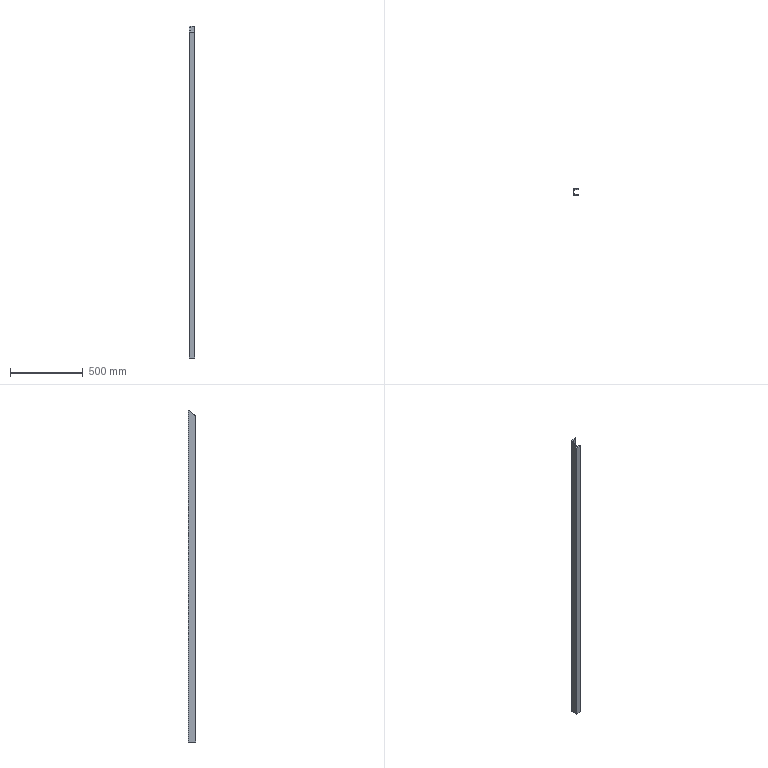Part | STEP file | DIN 1026-1 U 50 1785357157092 | 1 solid | 14 faces | box 38 x 50 x 2278 mm | volume 1606422 mm3 | plane 10 | cylinder 4 | commonest cylinder face diameters 7 x2 14 x2
STEP:
#1=CARTESIAN_POINT('',(5.,-10.418,2334.303));
#2=VERTEX_POINT('',#1);
#3=CARTESIAN_POINT('',(11.442,-17.395,2328.445));
#4=VERTEX_POINT('',#3);
#5=CARTESIAN_POINT('',(12.,-10.418,2334.303));
#6=DIRECTION('',(0.,-0.643,0.7659));
#7=DIRECTION('',(0.,-0.7659,-0.643));
#8=AXIS2_PLACEMENT_3D('',#5,#6,#7);
#9=ELLIPSE('',#8,9.14,7.);
#10=EDGE_CURVE('',#2,#4,#9,.T.);
#11=ORIENTED_EDGE('',*,*,#10,.F.);
#12=CARTESIAN_POINT('',(5.,10.418,2351.795));
#13=VERTEX_POINT('',#12);
#14=CARTESIAN_POINT('',(5.,-1153.83,1374.368));
#15=DIRECTION('',(0.,-0.7659,-0.643));
#16=VECTOR('',#15,10.);
#17=LINE('',#14,#16);
#18=EDGE_CURVE('',#13,#2,#17,.T.);
#19=ORIENTED_EDGE('',*,*,#18,.F.);
#20=CARTESIAN_POINT('',(11.442,17.395,2357.653));
#21=VERTEX_POINT('',#20);
#22=CARTESIAN_POINT('',(12.,10.418,2351.795));
#23=DIRECTION('',(0.,-0.643,0.7659));
#24=DIRECTION('',(0.,0.7659,0.643));
#25=AXIS2_PLACEMENT_3D('',#22,#23,#24);
#26=ELLIPSE('',#25,9.14,7.);
#27=EDGE_CURVE('',#21,#13,#26,.T.);
#28=ORIENTED_EDGE('',*,*,#27,.F.);
#29=CARTESIAN_POINT('',(34.779,19.262,2359.22));
#30=VERTEX_POINT('',#29);
#31=CARTESIAN_POINT('',(-139.927,5.286,2347.486));
#32=DIRECTION('',(-0.9946,-0.07957,-0.0668));
#33=VECTOR('',#32,10.);
#34=LINE('',#31,#33);
#35=EDGE_CURVE('',#30,#21,#34,.T.);
#36=ORIENTED_EDGE('',*,*,#35,.F.);
#37=CARTESIAN_POINT('',(38.,22.751,2362.149));
#38=VERTEX_POINT('',#37);
#39=CARTESIAN_POINT('',(34.5,22.751,2362.149));
#40=DIRECTION('',(0.,0.643,-0.7659));
#41=DIRECTION('',(0.,0.7659,0.643));
#42=AXIS2_PLACEMENT_3D('',#39,#40,#41);
#43=ELLIPSE('',#42,4.57,3.5);
#44=EDGE_CURVE('',#38,#30,#43,.T.);
#45=ORIENTED_EDGE('',*,*,#44,.F.);
#46=CARTESIAN_POINT('',(38.,25.,2364.037));
#47=VERTEX_POINT('',#46);
#48=CARTESIAN_POINT('',(38.,-1146.498,1380.523));
#49=DIRECTION('',(0.,-0.7659,-0.643));
#50=VECTOR('',#49,10.);
#51=LINE('',#48,#50);
#52=EDGE_CURVE('',#47,#38,#51,.T.);
#53=ORIENTED_EDGE('',*,*,#52,.F.);
#54=CARTESIAN_POINT('',(0.,25.,2364.037));
#55=VERTEX_POINT('',#54);
#56=CARTESIAN_POINT('',(9.5,25.,2364.037));
#57=DIRECTION('',(1.,0.,0.));
#58=VECTOR('',#57,10.);
#59=LINE('',#56,#58);
#60=EDGE_CURVE('',#55,#47,#59,.T.);
#61=ORIENTED_EDGE('',*,*,#60,.F.);
#62=CARTESIAN_POINT('',(0.,-25.,2322.06));
#63=VERTEX_POINT('',#62);
#64=CARTESIAN_POINT('',(0.,-1153.83,1374.368));
#65=DIRECTION('',(0.,0.7659,0.643));
#66=VECTOR('',#65,10.);
#67=LINE('',#64,#66);
#68=EDGE_CURVE('',#63,#55,#67,.T.);
#69=ORIENTED_EDGE('',*,*,#68,.F.);
#70=CARTESIAN_POINT('',(38.,-25.,2322.06));
#71=VERTEX_POINT('',#70);
#72=CARTESIAN_POINT('',(19.,-25.,2322.06));
#73=DIRECTION('',(-1.,0.,0.));
#74=VECTOR('',#73,10.);
#75=LINE('',#72,#74);
#76=EDGE_CURVE('',#71,#63,#75,.T.);
#77=ORIENTED_EDGE('',*,*,#76,.F.);
#78=CARTESIAN_POINT('',(38.,-22.751,2323.948));
#79=VERTEX_POINT('',#78);
#80=CARTESIAN_POINT('',(38.,-1160.503,1368.766));
#81=DIRECTION('',(0.,-0.7659,-0.643));
#82=VECTOR('',#81,10.);
#83=LINE('',#80,#82);
#84=EDGE_CURVE('',#79,#71,#83,.T.);
#85=ORIENTED_EDGE('',*,*,#84,.F.);
#86=CARTESIAN_POINT('',(34.779,-19.262,2326.877));
#87=VERTEX_POINT('',#86);
#88=CARTESIAN_POINT('',(34.5,-22.751,2323.948));
#89=DIRECTION('',(0.,0.643,-0.7659));
#90=DIRECTION('',(0.,-0.7659,-0.643));
#91=AXIS2_PLACEMENT_3D('',#88,#89,#90);
#92=ELLIPSE('',#91,4.57,3.5);
#93=EDGE_CURVE('',#87,#79,#92,.T.);
#94=ORIENTED_EDGE('',*,*,#93,.F.);
#95=CARTESIAN_POINT('',(159.791,-29.263,2318.481));
#96=DIRECTION('',(0.9946,-0.07957,-0.0668));
#97=VECTOR('',#96,10.);
#98=LINE('',#95,#97);
#99=EDGE_CURVE('',#4,#87,#98,.T.);
#100=ORIENTED_EDGE('',*,*,#99,.F.);
#101=EDGE_LOOP('',(#11,#19,#28,#36,#45,#53,#61,#69,#77,#85,#94,#100));
#102=FACE_OUTER_BOUND('',#101,.T.);
#103=CARTESIAN_POINT('',(0.,-1153.83,1374.368));
#104=DIRECTION('',(0.,0.643,-0.7659));
#105=DIRECTION('',(-1.,0.,0.));
#106=AXIS2_PLACEMENT_3D('',#103,#104,#105);
#107=PLANE('',#106);
#108=ADVANCED_FACE('',(#102),#107,.F.);
#109=ORIENTED_EDGE('',*,*,#52,.T.);
#110=CARTESIAN_POINT('',(38.,22.751,86.4));
#111=VERTEX_POINT('',#110);
#112=CARTESIAN_POINT('',(38.,22.751,0.));
#113=DIRECTION('',(0.,0.,1.));
#114=VECTOR('',#113,10.);
#115=LINE('',#112,#114);
#116=EDGE_CURVE('',#111,#38,#115,.T.);
#117=ORIENTED_EDGE('',*,*,#116,.F.);
#118=CARTESIAN_POINT('',(38.,25.,86.4));
#119=VERTEX_POINT('',#118);
#120=CARTESIAN_POINT('',(38.,12.5,86.4));
#121=DIRECTION('',(0.,-1.,0.));
#122=VECTOR('',#121,10.);
#123=LINE('',#120,#122);
#124=EDGE_CURVE('',#119,#111,#123,.T.);
#125=ORIENTED_EDGE('',*,*,#124,.F.);
#126=CARTESIAN_POINT('',(38.,25.,0.));
#127=DIRECTION('',(0.,0.,1.));
#128=VECTOR('',#127,10.);
#129=LINE('',#126,#128);
#130=EDGE_CURVE('',#119,#47,#129,.T.);
#131=ORIENTED_EDGE('',*,*,#130,.T.);
#132=EDGE_LOOP('',(#109,#117,#125,#131));
#133=FACE_OUTER_BOUND('',#132,.T.);
#134=CARTESIAN_POINT('',(38.,25.,0.));
#135=DIRECTION('',(1.,0.,0.));
#136=DIRECTION('',(0.,0.,-1.));
#137=AXIS2_PLACEMENT_3D('',#134,#135,#136);
#138=PLANE('',#137);
#139=ADVANCED_FACE('',(#133),#138,.T.);
#140=ORIENTED_EDGE('',*,*,#44,.T.);
#141=CARTESIAN_POINT('',(34.779,19.262,86.4));
#142=VERTEX_POINT('',#141);
#143=CARTESIAN_POINT('',(34.779,19.262,0.));
#144=DIRECTION('',(0.,0.,1.));
#145=VECTOR('',#144,10.);
#146=LINE('',#143,#145);
#147=EDGE_CURVE('',#142,#30,#146,.T.);
#148=ORIENTED_EDGE('',*,*,#147,.F.);
#149=CARTESIAN_POINT('',(34.5,22.751,86.4));
#150=DIRECTION('',(0.,0.,-1.));
#151=DIRECTION('',(-0.07975,0.9968,0.));
#152=AXIS2_PLACEMENT_3D('',#149,#150,#151);
#153=CIRCLE('',#152,3.5);
#154=EDGE_CURVE('',#111,#142,#153,.T.);
#155=ORIENTED_EDGE('',*,*,#154,.F.);
#156=ORIENTED_EDGE('',*,*,#116,.T.);
#157=EDGE_LOOP('',(#140,#148,#155,#156));
#158=FACE_OUTER_BOUND('',#157,.T.);
#159=CARTESIAN_POINT('',(34.5,22.751,0.));
#160=DIRECTION('',(0.,0.,1.));
#161=DIRECTION('',(-0.07975,0.9968,0.));
#162=AXIS2_PLACEMENT_3D('',#159,#160,#161);
#163=CYLINDRICAL_SURFACE('',#162,3.5);
#164=ADVANCED_FACE('',(#158),#163,.T.);
#165=ORIENTED_EDGE('',*,*,#35,.T.);
#166=CARTESIAN_POINT('',(11.442,17.395,86.4));
#167=VERTEX_POINT('',#166);
#168=CARTESIAN_POINT('',(11.442,17.395,0.));
#169=DIRECTION('',(0.,0.,1.));
#170=VECTOR('',#169,10.);
#171=LINE('',#168,#170);
#172=EDGE_CURVE('',#167,#21,#171,.T.);
#173=ORIENTED_EDGE('',*,*,#172,.F.);
#174=CARTESIAN_POINT('',(26.174,18.574,86.4));
#175=DIRECTION('',(-0.9968,-0.07975,0.));
#176=VECTOR('',#175,10.);
#177=LINE('',#174,#176);
#178=EDGE_CURVE('',#142,#167,#177,.T.);
#179=ORIENTED_EDGE('',*,*,#178,.F.);
#180=ORIENTED_EDGE('',*,*,#147,.T.);
#181=EDGE_LOOP('',(#165,#173,#179,#180));
#182=FACE_OUTER_BOUND('',#181,.T.);
#183=CARTESIAN_POINT('',(34.779,19.262,0.));
#184=DIRECTION('',(0.07975,-0.9968,0.));
#185=DIRECTION('',(0.,0.,-1.));
#186=AXIS2_PLACEMENT_3D('',#183,#184,#185);
#187=PLANE('',#186);
#188=ADVANCED_FACE('',(#182),#187,.T.);
#189=ORIENTED_EDGE('',*,*,#27,.T.);
#190=CARTESIAN_POINT('',(5.,10.418,86.4));
#191=VERTEX_POINT('',#190);
#192=CARTESIAN_POINT('',(5.,10.418,0.));
#193=DIRECTION('',(0.,0.,1.));
#194=VECTOR('',#193,10.);
#195=LINE('',#192,#194);
#196=EDGE_CURVE('',#191,#13,#195,.T.);
#197=ORIENTED_EDGE('',*,*,#196,.F.);
#198=CARTESIAN_POINT('',(12.,10.418,86.4));
#199=DIRECTION('',(0.,0.,1.));
#200=DIRECTION('',(-0.07975,0.9968,0.));
#201=AXIS2_PLACEMENT_3D('',#198,#199,#200);
#202=CIRCLE('',#201,7.);
#203=EDGE_CURVE('',#167,#191,#202,.T.);
#204=ORIENTED_EDGE('',*,*,#203,.F.);
#205=ORIENTED_EDGE('',*,*,#172,.T.);
#206=EDGE_LOOP('',(#189,#197,#204,#205));
#207=FACE_OUTER_BOUND('',#206,.T.);
#208=CARTESIAN_POINT('',(12.,10.418,0.));
#209=DIRECTION('',(0.,0.,1.));
#210=DIRECTION('',(-0.07975,0.9968,0.));
#211=AXIS2_PLACEMENT_3D('',#208,#209,#210);
#212=CYLINDRICAL_SURFACE('',#211,7.);
#213=ADVANCED_FACE('',(#207),#212,.F.);
#214=ORIENTED_EDGE('',*,*,#18,.T.);
#215=CARTESIAN_POINT('',(5.,-10.418,86.4));
#216=VERTEX_POINT('',#215);
#217=CARTESIAN_POINT('',(5.,-10.418,0.));
#218=DIRECTION('',(0.,0.,1.));
#219=VECTOR('',#218,10.);
#220=LINE('',#217,#219);
#221=EDGE_CURVE('',#216,#2,#220,.T.);
#222=ORIENTED_EDGE('',*,*,#221,.F.);
#223=CARTESIAN_POINT('',(5.,0.,86.4));
#224=DIRECTION('',(0.,-1.,0.));
#225=VECTOR('',#224,10.);
#226=LINE('',#223,#225);
#227=EDGE_CURVE('',#191,#216,#226,.T.);
#228=ORIENTED_EDGE('',*,*,#227,.F.);
#229=ORIENTED_EDGE('',*,*,#196,.T.);
#230=EDGE_LOOP('',(#214,#222,#228,#229));
#231=FACE_OUTER_BOUND('',#230,.T.);
#232=CARTESIAN_POINT('',(5.,0.,0.));
#233=DIRECTION('',(1.,0.,0.));
#234=DIRECTION('',(0.,0.,-1.));
#235=AXIS2_PLACEMENT_3D('',#232,#233,#234);
#236=PLANE('',#235);
#237=ADVANCED_FACE('',(#231),#236,.T.);
#238=ORIENTED_EDGE('',*,*,#10,.T.);
#239=CARTESIAN_POINT('',(11.442,-17.395,86.4));
#240=VERTEX_POINT('',#239);
#241=CARTESIAN_POINT('',(11.442,-17.395,0.));
#242=DIRECTION('',(0.,0.,1.));
#243=VECTOR('',#242,10.);
#244=LINE('',#241,#243);
#245=EDGE_CURVE('',#240,#4,#244,.T.);
#246=ORIENTED_EDGE('',*,*,#245,.F.);
#247=CARTESIAN_POINT('',(12.,-10.418,86.4));
#248=DIRECTION('',(0.,0.,1.));
#249=DIRECTION('',(-1.,0.,0.));
#250=AXIS2_PLACEMENT_3D('',#247,#248,#249);
#251=CIRCLE('',#250,7.);
#252=EDGE_CURVE('',#216,#240,#251,.T.);
#253=ORIENTED_EDGE('',*,*,#252,.F.);
#254=ORIENTED_EDGE('',*,*,#221,.T.);
#255=EDGE_LOOP('',(#238,#246,#253,#254));
#256=FACE_OUTER_BOUND('',#255,.T.);
#257=CARTESIAN_POINT('',(12.,-10.418,0.));
#258=DIRECTION('',(0.,0.,1.));
#259=DIRECTION('',(-1.,0.,0.));
#260=AXIS2_PLACEMENT_3D('',#257,#258,#259);
#261=CYLINDRICAL_SURFACE('',#260,7.);
#262=ADVANCED_FACE('',(#256),#261,.F.);
#263=ORIENTED_EDGE('',*,*,#99,.T.);
#264=CARTESIAN_POINT('',(34.779,-19.262,86.4));
#265=VERTEX_POINT('',#264);
#266=CARTESIAN_POINT('',(34.779,-19.262,0.));
#267=DIRECTION('',(0.,0.,1.));
#268=VECTOR('',#267,10.);
#269=LINE('',#266,#268);
#270=EDGE_CURVE('',#265,#87,#269,.T.);
#271=ORIENTED_EDGE('',*,*,#270,.F.);
#272=CARTESIAN_POINT('',(14.505,-17.64,86.4));
#273=DIRECTION('',(0.9968,-0.07975,0.));
#274=VECTOR('',#273,10.);
#275=LINE('',#272,#274);
#276=EDGE_CURVE('',#240,#265,#275,.T.);
#277=ORIENTED_EDGE('',*,*,#276,.F.);
#278=ORIENTED_EDGE('',*,*,#245,.T.);
#279=EDGE_LOOP('',(#263,#271,#277,#278));
#280=FACE_OUTER_BOUND('',#279,.T.);
#281=CARTESIAN_POINT('',(11.442,-17.395,0.));
#282=DIRECTION('',(0.07975,0.9968,0.));
#283=DIRECTION('',(0.,0.,1.));
#284=AXIS2_PLACEMENT_3D('',#281,#282,#283);
#285=PLANE('',#284);
#286=ADVANCED_FACE('',(#280),#285,.T.);
#287=ORIENTED_EDGE('',*,*,#93,.T.);
#288=CARTESIAN_POINT('',(38.,-22.751,86.4));
#289=VERTEX_POINT('',#288);
#290=CARTESIAN_POINT('',(38.,-22.751,0.));
#291=DIRECTION('',(0.,0.,1.));
#292=VECTOR('',#291,10.);
#293=LINE('',#290,#292);
#294=EDGE_CURVE('',#289,#79,#293,.T.);
#295=ORIENTED_EDGE('',*,*,#294,.F.);
#296=CARTESIAN_POINT('',(34.5,-22.751,86.4));
#297=DIRECTION('',(0.,0.,-1.));
#298=DIRECTION('',(-1.,0.,0.));
#299=AXIS2_PLACEMENT_3D('',#296,#297,#298);
#300=CIRCLE('',#299,3.5);
#301=EDGE_CURVE('',#265,#289,#300,.T.);
#302=ORIENTED_EDGE('',*,*,#301,.F.);
#303=ORIENTED_EDGE('',*,*,#270,.T.);
#304=EDGE_LOOP('',(#287,#295,#302,#303));
#305=FACE_OUTER_BOUND('',#304,.T.);
#306=CARTESIAN_POINT('',(34.5,-22.751,0.));
#307=DIRECTION('',(0.,0.,1.));
#308=DIRECTION('',(-1.,0.,0.));
#309=AXIS2_PLACEMENT_3D('',#306,#307,#308);
#310=CYLINDRICAL_SURFACE('',#309,3.5);
#311=ADVANCED_FACE('',(#305),#310,.T.);
#312=ORIENTED_EDGE('',*,*,#84,.T.);
#313=CARTESIAN_POINT('',(38.,-25.,86.4));
#314=VERTEX_POINT('',#313);
#315=CARTESIAN_POINT('',(38.,-25.,0.));
#316=DIRECTION('',(0.,0.,1.));
#317=VECTOR('',#316,10.);
#318=LINE('',#315,#317);
#319=EDGE_CURVE('',#314,#71,#318,.T.);
#320=ORIENTED_EDGE('',*,*,#319,.F.);
#321=CARTESIAN_POINT('',(38.,-11.376,86.4));
#322=DIRECTION('',(0.,-1.,0.));
#323=VECTOR('',#322,10.);
#324=LINE('',#321,#323);
#325=EDGE_CURVE('',#289,#314,#324,.T.);
#326=ORIENTED_EDGE('',*,*,#325,.F.);
#327=ORIENTED_EDGE('',*,*,#294,.T.);
#328=EDGE_LOOP('',(#312,#320,#326,#327));
#329=FACE_OUTER_BOUND('',#328,.T.);
#330=CARTESIAN_POINT('',(38.,-22.751,0.));
#331=DIRECTION('',(1.,0.,0.));
#332=DIRECTION('',(0.,0.,-1.));
#333=AXIS2_PLACEMENT_3D('',#330,#331,#332);
#334=PLANE('',#333);
#335=ADVANCED_FACE('',(#329),#334,.T.);
#336=ORIENTED_EDGE('',*,*,#76,.T.);
#337=CARTESIAN_POINT('',(0.,-25.,86.4));
#338=VERTEX_POINT('',#337);
#339=CARTESIAN_POINT('',(0.,-25.,0.));
#340=DIRECTION('',(0.,0.,1.));
#341=VECTOR('',#340,10.);
#342=LINE('',#339,#341);
#343=EDGE_CURVE('',#338,#63,#342,.T.);
#344=ORIENTED_EDGE('',*,*,#343,.F.);
#345=CARTESIAN_POINT('',(28.5,-25.,86.4));
#346=DIRECTION('',(-1.,0.,0.));
#347=VECTOR('',#346,10.);
#348=LINE('',#345,#347);
#349=EDGE_CURVE('',#314,#338,#348,.T.);
#350=ORIENTED_EDGE('',*,*,#349,.F.);
#351=ORIENTED_EDGE('',*,*,#319,.T.);
#352=EDGE_LOOP('',(#336,#344,#350,#351));
#353=FACE_OUTER_BOUND('',#352,.T.);
#354=CARTESIAN_POINT('',(38.,-25.,0.));
#355=DIRECTION('',(0.,-1.,0.));
#356=DIRECTION('',(0.,0.,-1.));
#357=AXIS2_PLACEMENT_3D('',#354,#355,#356);
#358=PLANE('',#357);
#359=ADVANCED_FACE('',(#353),#358,.T.);
#360=ORIENTED_EDGE('',*,*,#68,.T.);
#361=CARTESIAN_POINT('',(0.,25.,86.4));
#362=VERTEX_POINT('',#361);
#363=CARTESIAN_POINT('',(0.,25.,0.));
#364=DIRECTION('',(0.,0.,1.));
#365=VECTOR('',#364,10.);
#366=LINE('',#363,#365);
#367=EDGE_CURVE('',#362,#55,#366,.T.);
#368=ORIENTED_EDGE('',*,*,#367,.F.);
#369=CARTESIAN_POINT('',(0.,0.,86.4));
#370=DIRECTION('',(0.,1.,0.));
#371=VECTOR('',#370,10.);
#372=LINE('',#369,#371);
#373=EDGE_CURVE('',#338,#362,#372,.T.);
#374=ORIENTED_EDGE('',*,*,#373,.F.);
#375=ORIENTED_EDGE('',*,*,#343,.T.);
#376=EDGE_LOOP('',(#360,#368,#374,#375));
#377=FACE_OUTER_BOUND('',#376,.T.);
#378=CARTESIAN_POINT('',(0.,0.,0.));
#379=DIRECTION('',(-1.,0.,0.));
#380=DIRECTION('',(0.,0.,1.));
#381=AXIS2_PLACEMENT_3D('',#378,#379,#380);
#382=PLANE('',#381);
#383=ADVANCED_FACE('',(#377),#382,.T.);
#384=ORIENTED_EDGE('',*,*,#60,.T.);
#385=ORIENTED_EDGE('',*,*,#130,.F.);
#386=CARTESIAN_POINT('',(9.5,25.,86.4));
#387=DIRECTION('',(1.,0.,0.));
#388=VECTOR('',#387,10.);
#389=LINE('',#386,#388);
#390=EDGE_CURVE('',#362,#119,#389,.T.);
#391=ORIENTED_EDGE('',*,*,#390,.F.);
#392=ORIENTED_EDGE('',*,*,#367,.T.);
#393=EDGE_LOOP('',(#384,#385,#391,#392));
#394=FACE_OUTER_BOUND('',#393,.T.);
#395=CARTESIAN_POINT('',(0.,25.,0.));
#396=DIRECTION('',(0.,1.,0.));
#397=DIRECTION('',(0.,0.,1.));
#398=AXIS2_PLACEMENT_3D('',#395,#396,#397);
#399=PLANE('',#398);
#400=ADVANCED_FACE('',(#394),#399,.T.);
#401=ORIENTED_EDGE('',*,*,#390,.T.);
#402=ORIENTED_EDGE('',*,*,#124,.T.);
#403=ORIENTED_EDGE('',*,*,#154,.T.);
#404=ORIENTED_EDGE('',*,*,#178,.T.);
#405=ORIENTED_EDGE('',*,*,#203,.T.);
#406=ORIENTED_EDGE('',*,*,#227,.T.);
#407=ORIENTED_EDGE('',*,*,#252,.T.);
#408=ORIENTED_EDGE('',*,*,#276,.T.);
#409=ORIENTED_EDGE('',*,*,#301,.T.);
#410=ORIENTED_EDGE('',*,*,#325,.T.);
#411=ORIENTED_EDGE('',*,*,#349,.T.);
#412=ORIENTED_EDGE('',*,*,#373,.T.);
#413=EDGE_LOOP('',(#401,#402,#403,#404,#405,#406,#407,#408,#409,#410,#411,#412));
#414=FACE_OUTER_BOUND('',#413,.T.);
#415=CARTESIAN_POINT('',(19.,0.,86.4));
#416=DIRECTION('',(0.,0.,1.));
#417=DIRECTION('',(1.,0.,0.));
#418=AXIS2_PLACEMENT_3D('',#415,#416,#417);
#419=PLANE('',#418);
#420=ADVANCED_FACE('',(#414),#419,.F.);
#421=CLOSED_SHELL('',(#108,#139,#164,#188,#213,#237,#262,#286,#311,#335,#359,#383,#400,#420));
#422=MANIFOLD_SOLID_BREP('',#421);
#423=(LENGTH_UNIT()NAMED_UNIT(*)SI_UNIT(.MILLI.,.METRE.));
#424=UNCERTAINTY_MEASURE_WITH_UNIT(LENGTH_MEASURE(0.01),#423,'','');
#425=(NAMED_UNIT(*)PLANE_ANGLE_UNIT()SI_UNIT($,.RADIAN.));
#426=(NAMED_UNIT(*)SI_UNIT($,.STERADIAN.)SOLID_ANGLE_UNIT());
#427=(GEOMETRIC_REPRESENTATION_CONTEXT(3)GLOBAL_UNCERTAINTY_ASSIGNED_CONTEXT((#424))GLOBAL_UNIT_ASSIGNED_CONTEXT((#423,#425,#426))REPRESENTATION_CONTEXT('',''));
#428=ADVANCED_BREP_SHAPE_REPRESENTATION('',(#422),#427);